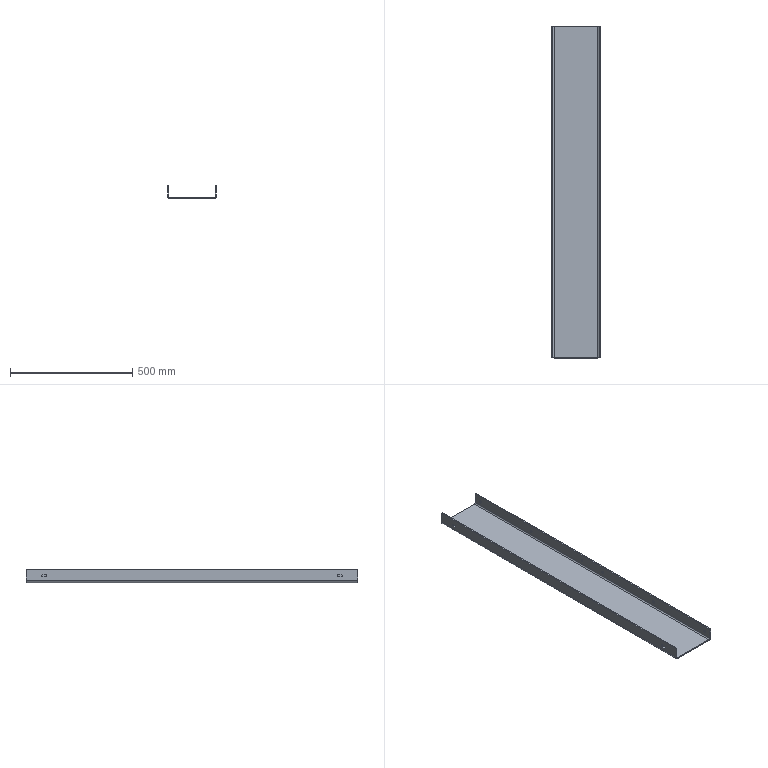Part | STEP file | VD-SYL0380DJ1006_1_1-4_VD-SYL03 | 1 solid | 34 faces | box 200 x 1360 x 55 mm | volume 1991838 mm3 | cylinder 20 | plane 14 | commonest cylinder face diameters 10.5 x12 10 x6 20 x2
STEP:
#1=CARTESIAN_POINT('',(95.,-60.,23.75));
#2=VERTEX_POINT('',#1);
#3=CARTESIAN_POINT('',(100.,-60.,23.75));
#4=VERTEX_POINT('',#3);
#5=CARTESIAN_POINT('',(95.,-60.,23.75));
#6=DIRECTION('',(1.,0.,0.));
#7=VECTOR('',#6,1000.);
#8=LINE('',#5,#7);
#9=EDGE_CURVE('',#2,#4,#8,.T.);
#10=ORIENTED_EDGE('',*,*,#9,.F.);
#11=CARTESIAN_POINT('',(95.,-60.,34.25));
#12=VERTEX_POINT('',#11);
#13=CARTESIAN_POINT('',(95.,-60.,29.));
#14=DIRECTION('',(1.,0.,0.));
#15=DIRECTION('',(0.,0.,1.));
#16=AXIS2_PLACEMENT_3D('',#13,#14,#15);
#17=CIRCLE('',#16,5.25);
#18=EDGE_CURVE('',#12,#2,#17,.T.);
#19=ORIENTED_EDGE('',*,*,#18,.F.);
#20=CARTESIAN_POINT('',(100.,-60.,34.25));
#21=VERTEX_POINT('',#20);
#22=CARTESIAN_POINT('',(95.,-60.,34.25));
#23=DIRECTION('',(1.,0.,0.));
#24=VECTOR('',#23,1000.);
#25=LINE('',#22,#24);
#26=EDGE_CURVE('',#12,#21,#25,.T.);
#27=ORIENTED_EDGE('',*,*,#26,.T.);
#28=CARTESIAN_POINT('',(100.,-60.,29.));
#29=DIRECTION('',(-1.,0.,0.));
#30=DIRECTION('',(0.,0.,-1.));
#31=AXIS2_PLACEMENT_3D('',#28,#29,#30);
#32=CIRCLE('',#31,5.25);
#33=EDGE_CURVE('',#4,#21,#32,.T.);
#34=ORIENTED_EDGE('',*,*,#33,.F.);
#35=EDGE_LOOP('',(#10,#19,#27,#34));
#36=FACE_OUTER_BOUND('',#35,.T.);
#37=CARTESIAN_POINT('',(97.5,-60.,29.));
#38=DIRECTION('',(-1.,0.,0.));
#39=DIRECTION('',(0.,0.,1.));
#40=AXIS2_PLACEMENT_3D('',#37,#38,#39);
#41=CYLINDRICAL_SURFACE('',#40,5.25);
#42=ADVANCED_FACE('',(#36),#41,.F.);
#43=CARTESIAN_POINT('',(100.,-60.,29.));
#44=DIRECTION('',(-1.,0.,0.));
#45=DIRECTION('',(0.,0.,1.));
#46=AXIS2_PLACEMENT_3D('',#43,#44,#45);
#47=CIRCLE('',#46,5.25);
#48=EDGE_CURVE('',#21,#4,#47,.T.);
#49=ORIENTED_EDGE('',*,*,#48,.F.);
#50=ORIENTED_EDGE('',*,*,#26,.F.);
#51=CARTESIAN_POINT('',(95.,-60.,29.));
#52=DIRECTION('',(1.,0.,0.));
#53=DIRECTION('',(0.,0.,-1.));
#54=AXIS2_PLACEMENT_3D('',#51,#52,#53);
#55=CIRCLE('',#54,5.25);
#56=EDGE_CURVE('',#2,#12,#55,.T.);
#57=ORIENTED_EDGE('',*,*,#56,.F.);
#58=ORIENTED_EDGE('',*,*,#9,.T.);
#59=EDGE_LOOP('',(#49,#50,#57,#58));
#60=FACE_OUTER_BOUND('',#59,.T.);
#61=CARTESIAN_POINT('',(97.5,-60.,29.));
#62=DIRECTION('',(-1.,0.,0.));
#63=DIRECTION('',(0.,0.,1.));
#64=AXIS2_PLACEMENT_3D('',#61,#62,#63);
#65=CYLINDRICAL_SURFACE('',#64,5.25);
#66=ADVANCED_FACE('',(#60),#65,.F.);
#67=CARTESIAN_POINT('',(95.,-355.,23.75));
#68=VERTEX_POINT('',#67);
#69=CARTESIAN_POINT('',(100.,-355.,23.75));
#70=VERTEX_POINT('',#69);
#71=CARTESIAN_POINT('',(95.,-355.,23.75));
#72=DIRECTION('',(1.,0.,0.));
#73=VECTOR('',#72,1000.);
#74=LINE('',#71,#73);
#75=EDGE_CURVE('',#68,#70,#74,.T.);
#76=ORIENTED_EDGE('',*,*,#75,.F.);
#77=CARTESIAN_POINT('',(95.,-355.,34.25));
#78=VERTEX_POINT('',#77);
#79=CARTESIAN_POINT('',(95.,-355.,29.));
#80=DIRECTION('',(1.,0.,0.));
#81=DIRECTION('',(0.,0.,1.));
#82=AXIS2_PLACEMENT_3D('',#79,#80,#81);
#83=CIRCLE('',#82,5.25);
#84=EDGE_CURVE('',#78,#68,#83,.T.);
#85=ORIENTED_EDGE('',*,*,#84,.F.);
#86=CARTESIAN_POINT('',(100.,-355.,34.25));
#87=VERTEX_POINT('',#86);
#88=CARTESIAN_POINT('',(95.,-355.,34.25));
#89=DIRECTION('',(1.,0.,0.));
#90=VECTOR('',#89,1000.);
#91=LINE('',#88,#90);
#92=EDGE_CURVE('',#78,#87,#91,.T.);
#93=ORIENTED_EDGE('',*,*,#92,.T.);
#94=CARTESIAN_POINT('',(100.,-355.,29.));
#95=DIRECTION('',(-1.,0.,0.));
#96=DIRECTION('',(0.,0.,-1.));
#97=AXIS2_PLACEMENT_3D('',#94,#95,#96);
#98=CIRCLE('',#97,5.25);
#99=EDGE_CURVE('',#70,#87,#98,.T.);
#100=ORIENTED_EDGE('',*,*,#99,.F.);
#101=EDGE_LOOP('',(#76,#85,#93,#100));
#102=FACE_OUTER_BOUND('',#101,.T.);
#103=CARTESIAN_POINT('',(97.5,-355.,29.));
#104=DIRECTION('',(-1.,0.,0.));
#105=DIRECTION('',(0.,0.,1.));
#106=AXIS2_PLACEMENT_3D('',#103,#104,#105);
#107=CYLINDRICAL_SURFACE('',#106,5.25);
#108=ADVANCED_FACE('',(#102),#107,.F.);
#109=CARTESIAN_POINT('',(100.,-355.,29.));
#110=DIRECTION('',(-1.,0.,0.));
#111=DIRECTION('',(0.,0.,1.));
#112=AXIS2_PLACEMENT_3D('',#109,#110,#111);
#113=CIRCLE('',#112,5.25);
#114=EDGE_CURVE('',#87,#70,#113,.T.);
#115=ORIENTED_EDGE('',*,*,#114,.F.);
#116=ORIENTED_EDGE('',*,*,#92,.F.);
#117=CARTESIAN_POINT('',(95.,-355.,29.));
#118=DIRECTION('',(1.,0.,0.));
#119=DIRECTION('',(0.,0.,-1.));
#120=AXIS2_PLACEMENT_3D('',#117,#118,#119);
#121=CIRCLE('',#120,5.25);
#122=EDGE_CURVE('',#68,#78,#121,.T.);
#123=ORIENTED_EDGE('',*,*,#122,.F.);
#124=ORIENTED_EDGE('',*,*,#75,.T.);
#125=EDGE_LOOP('',(#115,#116,#123,#124));
#126=FACE_OUTER_BOUND('',#125,.T.);
#127=CARTESIAN_POINT('',(97.5,-355.,29.));
#128=DIRECTION('',(-1.,0.,0.));
#129=DIRECTION('',(0.,0.,1.));
#130=AXIS2_PLACEMENT_3D('',#127,#128,#129);
#131=CYLINDRICAL_SURFACE('',#130,5.25);
#132=ADVANCED_FACE('',(#126),#131,.F.);
#133=CARTESIAN_POINT('',(95.,-650.,23.75));
#134=VERTEX_POINT('',#133);
#135=CARTESIAN_POINT('',(100.,-650.,23.75));
#136=VERTEX_POINT('',#135);
#137=CARTESIAN_POINT('',(95.,-650.,23.75));
#138=DIRECTION('',(1.,0.,0.));
#139=VECTOR('',#138,1000.);
#140=LINE('',#137,#139);
#141=EDGE_CURVE('',#134,#136,#140,.T.);
#142=ORIENTED_EDGE('',*,*,#141,.F.);
#143=CARTESIAN_POINT('',(95.,-650.,34.25));
#144=VERTEX_POINT('',#143);
#145=CARTESIAN_POINT('',(95.,-650.,29.));
#146=DIRECTION('',(1.,0.,0.));
#147=DIRECTION('',(0.,0.,1.));
#148=AXIS2_PLACEMENT_3D('',#145,#146,#147);
#149=CIRCLE('',#148,5.25);
#150=EDGE_CURVE('',#144,#134,#149,.T.);
#151=ORIENTED_EDGE('',*,*,#150,.F.);
#152=CARTESIAN_POINT('',(100.,-650.,34.25));
#153=VERTEX_POINT('',#152);
#154=CARTESIAN_POINT('',(95.,-650.,34.25));
#155=DIRECTION('',(1.,0.,0.));
#156=VECTOR('',#155,1000.);
#157=LINE('',#154,#156);
#158=EDGE_CURVE('',#144,#153,#157,.T.);
#159=ORIENTED_EDGE('',*,*,#158,.T.);
#160=CARTESIAN_POINT('',(100.,-650.,29.));
#161=DIRECTION('',(-1.,0.,0.));
#162=DIRECTION('',(0.,0.,-1.));
#163=AXIS2_PLACEMENT_3D('',#160,#161,#162);
#164=CIRCLE('',#163,5.25);
#165=EDGE_CURVE('',#136,#153,#164,.T.);
#166=ORIENTED_EDGE('',*,*,#165,.F.);
#167=EDGE_LOOP('',(#142,#151,#159,#166));
#168=FACE_OUTER_BOUND('',#167,.T.);
#169=CARTESIAN_POINT('',(97.5,-650.,29.));
#170=DIRECTION('',(-1.,0.,0.));
#171=DIRECTION('',(0.,0.,1.));
#172=AXIS2_PLACEMENT_3D('',#169,#170,#171);
#173=CYLINDRICAL_SURFACE('',#172,5.25);
#174=ADVANCED_FACE('',(#168),#173,.F.);
#175=CARTESIAN_POINT('',(100.,-650.,29.));
#176=DIRECTION('',(-1.,0.,0.));
#177=DIRECTION('',(0.,0.,1.));
#178=AXIS2_PLACEMENT_3D('',#175,#176,#177);
#179=CIRCLE('',#178,5.25);
#180=EDGE_CURVE('',#153,#136,#179,.T.);
#181=ORIENTED_EDGE('',*,*,#180,.F.);
#182=ORIENTED_EDGE('',*,*,#158,.F.);
#183=CARTESIAN_POINT('',(95.,-650.,29.));
#184=DIRECTION('',(1.,0.,0.));
#185=DIRECTION('',(0.,0.,-1.));
#186=AXIS2_PLACEMENT_3D('',#183,#184,#185);
#187=CIRCLE('',#186,5.25);
#188=EDGE_CURVE('',#134,#144,#187,.T.);
#189=ORIENTED_EDGE('',*,*,#188,.F.);
#190=ORIENTED_EDGE('',*,*,#141,.T.);
#191=EDGE_LOOP('',(#181,#182,#189,#190));
#192=FACE_OUTER_BOUND('',#191,.T.);
#193=CARTESIAN_POINT('',(97.5,-650.,29.));
#194=DIRECTION('',(-1.,0.,0.));
#195=DIRECTION('',(0.,0.,1.));
#196=AXIS2_PLACEMENT_3D('',#193,#194,#195);
#197=CYLINDRICAL_SURFACE('',#196,5.25);
#198=ADVANCED_FACE('',(#192),#197,.F.);
#199=CARTESIAN_POINT('',(95.,60.,23.75));
#200=VERTEX_POINT('',#199);
#201=CARTESIAN_POINT('',(95.,60.,34.25));
#202=VERTEX_POINT('',#201);
#203=CARTESIAN_POINT('',(95.,60.,29.));
#204=DIRECTION('',(1.,0.,0.));
#205=DIRECTION('',(0.,0.,-1.));
#206=AXIS2_PLACEMENT_3D('',#203,#204,#205);
#207=CIRCLE('',#206,5.25);
#208=EDGE_CURVE('',#200,#202,#207,.T.);
#209=ORIENTED_EDGE('',*,*,#208,.F.);
#210=CARTESIAN_POINT('',(100.,60.,23.75));
#211=VERTEX_POINT('',#210);
#212=CARTESIAN_POINT('',(100.,60.,23.75));
#213=DIRECTION('',(-1.,0.,0.));
#214=VECTOR('',#213,1000.);
#215=LINE('',#212,#214);
#216=EDGE_CURVE('',#211,#200,#215,.T.);
#217=ORIENTED_EDGE('',*,*,#216,.F.);
#218=CARTESIAN_POINT('',(100.,60.,34.25));
#219=VERTEX_POINT('',#218);
#220=CARTESIAN_POINT('',(100.,60.,29.));
#221=DIRECTION('',(-1.,0.,0.));
#222=DIRECTION('',(0.,0.,1.));
#223=AXIS2_PLACEMENT_3D('',#220,#221,#222);
#224=CIRCLE('',#223,5.25);
#225=EDGE_CURVE('',#219,#211,#224,.T.);
#226=ORIENTED_EDGE('',*,*,#225,.F.);
#227=CARTESIAN_POINT('',(100.,60.,34.25));
#228=DIRECTION('',(-1.,0.,0.));
#229=VECTOR('',#228,1000.);
#230=LINE('',#227,#229);
#231=EDGE_CURVE('',#219,#202,#230,.T.);
#232=ORIENTED_EDGE('',*,*,#231,.T.);
#233=EDGE_LOOP('',(#209,#217,#226,#232));
#234=FACE_OUTER_BOUND('',#233,.T.);
#235=CARTESIAN_POINT('',(97.5,60.,29.));
#236=DIRECTION('',(1.,0.,0.));
#237=DIRECTION('',(0.,0.,-1.));
#238=AXIS2_PLACEMENT_3D('',#235,#236,#237);
#239=CYLINDRICAL_SURFACE('',#238,5.25);
#240=ADVANCED_FACE('',(#234),#239,.F.);
#241=ORIENTED_EDGE('',*,*,#231,.F.);
#242=CARTESIAN_POINT('',(100.,60.,29.));
#243=DIRECTION('',(-1.,0.,0.));
#244=DIRECTION('',(0.,0.,-1.));
#245=AXIS2_PLACEMENT_3D('',#242,#243,#244);
#246=CIRCLE('',#245,5.25);
#247=EDGE_CURVE('',#211,#219,#246,.T.);
#248=ORIENTED_EDGE('',*,*,#247,.F.);
#249=ORIENTED_EDGE('',*,*,#216,.T.);
#250=CARTESIAN_POINT('',(95.,60.,29.));
#251=DIRECTION('',(1.,0.,0.));
#252=DIRECTION('',(0.,0.,1.));
#253=AXIS2_PLACEMENT_3D('',#250,#251,#252);
#254=CIRCLE('',#253,5.25);
#255=EDGE_CURVE('',#202,#200,#254,.T.);
#256=ORIENTED_EDGE('',*,*,#255,.F.);
#257=EDGE_LOOP('',(#241,#248,#249,#256));
#258=FACE_OUTER_BOUND('',#257,.T.);
#259=CARTESIAN_POINT('',(97.5,60.,29.));
#260=DIRECTION('',(1.,0.,0.));
#261=DIRECTION('',(0.,0.,-1.));
#262=AXIS2_PLACEMENT_3D('',#259,#260,#261);
#263=CYLINDRICAL_SURFACE('',#262,5.25);
#264=ADVANCED_FACE('',(#258),#263,.F.);
#265=CARTESIAN_POINT('',(95.,355.,23.75));
#266=VERTEX_POINT('',#265);
#267=CARTESIAN_POINT('',(95.,355.,34.25));
#268=VERTEX_POINT('',#267);
#269=CARTESIAN_POINT('',(95.,355.,29.));
#270=DIRECTION('',(1.,0.,0.));
#271=DIRECTION('',(0.,0.,-1.));
#272=AXIS2_PLACEMENT_3D('',#269,#270,#271);
#273=CIRCLE('',#272,5.25);
#274=EDGE_CURVE('',#266,#268,#273,.T.);
#275=ORIENTED_EDGE('',*,*,#274,.F.);
#276=CARTESIAN_POINT('',(100.,355.,23.75));
#277=VERTEX_POINT('',#276);
#278=CARTESIAN_POINT('',(100.,355.,23.75));
#279=DIRECTION('',(-1.,0.,0.));
#280=VECTOR('',#279,1000.);
#281=LINE('',#278,#280);
#282=EDGE_CURVE('',#277,#266,#281,.T.);
#283=ORIENTED_EDGE('',*,*,#282,.F.);
#284=CARTESIAN_POINT('',(100.,355.,34.25));
#285=VERTEX_POINT('',#284);
#286=CARTESIAN_POINT('',(100.,355.,29.));
#287=DIRECTION('',(-1.,0.,0.));
#288=DIRECTION('',(0.,0.,1.));
#289=AXIS2_PLACEMENT_3D('',#286,#287,#288);
#290=CIRCLE('',#289,5.25);
#291=EDGE_CURVE('',#285,#277,#290,.T.);
#292=ORIENTED_EDGE('',*,*,#291,.F.);
#293=CARTESIAN_POINT('',(100.,355.,34.25));
#294=DIRECTION('',(-1.,0.,0.));
#295=VECTOR('',#294,1000.);
#296=LINE('',#293,#295);
#297=EDGE_CURVE('',#285,#268,#296,.T.);
#298=ORIENTED_EDGE('',*,*,#297,.T.);
#299=EDGE_LOOP('',(#275,#283,#292,#298));
#300=FACE_OUTER_BOUND('',#299,.T.);
#301=CARTESIAN_POINT('',(97.5,355.,29.));
#302=DIRECTION('',(1.,0.,0.));
#303=DIRECTION('',(0.,0.,-1.));
#304=AXIS2_PLACEMENT_3D('',#301,#302,#303);
#305=CYLINDRICAL_SURFACE('',#304,5.25);
#306=ADVANCED_FACE('',(#300),#305,.F.);
#307=ORIENTED_EDGE('',*,*,#297,.F.);
#308=CARTESIAN_POINT('',(100.,355.,29.));
#309=DIRECTION('',(-1.,0.,0.));
#310=DIRECTION('',(0.,0.,-1.));
#311=AXIS2_PLACEMENT_3D('',#308,#309,#310);
#312=CIRCLE('',#311,5.25);
#313=EDGE_CURVE('',#277,#285,#312,.T.);
#314=ORIENTED_EDGE('',*,*,#313,.F.);
#315=ORIENTED_EDGE('',*,*,#282,.T.);
#316=CARTESIAN_POINT('',(95.,355.,29.));
#317=DIRECTION('',(1.,0.,0.));
#318=DIRECTION('',(0.,0.,1.));
#319=AXIS2_PLACEMENT_3D('',#316,#317,#318);
#320=CIRCLE('',#319,5.25);
#321=EDGE_CURVE('',#268,#266,#320,.T.);
#322=ORIENTED_EDGE('',*,*,#321,.F.);
#323=EDGE_LOOP('',(#307,#314,#315,#322));
#324=FACE_OUTER_BOUND('',#323,.T.);
#325=CARTESIAN_POINT('',(97.5,355.,29.));
#326=DIRECTION('',(1.,0.,0.));
#327=DIRECTION('',(0.,0.,-1.));
#328=AXIS2_PLACEMENT_3D('',#325,#326,#327);
#329=CYLINDRICAL_SURFACE('',#328,5.25);
#330=ADVANCED_FACE('',(#324),#329,.F.);
#331=CARTESIAN_POINT('',(95.,650.,23.75));
#332=VERTEX_POINT('',#331);
#333=CARTESIAN_POINT('',(95.,650.,34.25));
#334=VERTEX_POINT('',#333);
#335=CARTESIAN_POINT('',(95.,650.,29.));
#336=DIRECTION('',(1.,0.,0.));
#337=DIRECTION('',(0.,0.,-1.));
#338=AXIS2_PLACEMENT_3D('',#335,#336,#337);
#339=CIRCLE('',#338,5.25);
#340=EDGE_CURVE('',#332,#334,#339,.T.);
#341=ORIENTED_EDGE('',*,*,#340,.F.);
#342=CARTESIAN_POINT('',(100.,650.,23.75));
#343=VERTEX_POINT('',#342);
#344=CARTESIAN_POINT('',(100.,650.,23.75));
#345=DIRECTION('',(-1.,0.,0.));
#346=VECTOR('',#345,1000.);
#347=LINE('',#344,#346);
#348=EDGE_CURVE('',#343,#332,#347,.T.);
#349=ORIENTED_EDGE('',*,*,#348,.F.);
#350=CARTESIAN_POINT('',(100.,650.,34.25));
#351=VERTEX_POINT('',#350);
#352=CARTESIAN_POINT('',(100.,650.,29.));
#353=DIRECTION('',(-1.,0.,0.));
#354=DIRECTION('',(0.,0.,1.));
#355=AXIS2_PLACEMENT_3D('',#352,#353,#354);
#356=CIRCLE('',#355,5.25);
#357=EDGE_CURVE('',#351,#343,#356,.T.);
#358=ORIENTED_EDGE('',*,*,#357,.F.);
#359=CARTESIAN_POINT('',(100.,650.,34.25));
#360=DIRECTION('',(-1.,0.,0.));
#361=VECTOR('',#360,1000.);
#362=LINE('',#359,#361);
#363=EDGE_CURVE('',#351,#334,#362,.T.);
#364=ORIENTED_EDGE('',*,*,#363,.T.);
#365=EDGE_LOOP('',(#341,#349,#358,#364));
#366=FACE_OUTER_BOUND('',#365,.T.);
#367=CARTESIAN_POINT('',(97.5,650.,29.));
#368=DIRECTION('',(1.,0.,0.));
#369=DIRECTION('',(0.,0.,-1.));
#370=AXIS2_PLACEMENT_3D('',#367,#368,#369);
#371=CYLINDRICAL_SURFACE('',#370,5.25);
#372=ADVANCED_FACE('',(#366),#371,.F.);
#373=ORIENTED_EDGE('',*,*,#363,.F.);
#374=CARTESIAN_POINT('',(100.,650.,29.));
#375=DIRECTION('',(-1.,0.,0.));
#376=DIRECTION('',(0.,0.,-1.));
#377=AXIS2_PLACEMENT_3D('',#374,#375,#376);
#378=CIRCLE('',#377,5.25);
#379=EDGE_CURVE('',#343,#351,#378,.T.);
#380=ORIENTED_EDGE('',*,*,#379,.F.);
#381=ORIENTED_EDGE('',*,*,#348,.T.);
#382=CARTESIAN_POINT('',(95.,650.,29.));
#383=DIRECTION('',(1.,0.,0.));
#384=DIRECTION('',(0.,0.,1.));
#385=AXIS2_PLACEMENT_3D('',#382,#383,#384);
#386=CIRCLE('',#385,5.25);
#387=EDGE_CURVE('',#334,#332,#386,.T.);
#388=ORIENTED_EDGE('',*,*,#387,.F.);
#389=EDGE_LOOP('',(#373,#380,#381,#388));
#390=FACE_OUTER_BOUND('',#389,.T.);
#391=CARTESIAN_POINT('',(97.5,650.,29.));
#392=DIRECTION('',(1.,0.,0.));
#393=DIRECTION('',(0.,0.,-1.));
#394=AXIS2_PLACEMENT_3D('',#391,#392,#393);
#395=CYLINDRICAL_SURFACE('',#394,5.25);
#396=ADVANCED_FACE('',(#390),#395,.F.);
#397=CARTESIAN_POINT('',(-95.,-601.,33.5));
#398=VERTEX_POINT('',#397);
#399=CARTESIAN_POINT('',(-100.,-601.,33.5));
#400=VERTEX_POINT('',#399);
#401=CARTESIAN_POINT('',(-95.,-601.,33.5));
#402=DIRECTION('',(-1.,0.,0.));
#403=VECTOR('',#402,1000.);
#404=LINE('',#401,#403);
#405=EDGE_CURVE('',#398,#400,#404,.T.);
#406=ORIENTED_EDGE('',*,*,#405,.T.);
#407=CARTESIAN_POINT('',(-100.,-601.,23.5));
#408=VERTEX_POINT('',#407);
#409=CARTESIAN_POINT('',(-100.,-601.,28.5));
#410=DIRECTION('',(1.,0.,0.));
#411=DIRECTION('',(0.,0.,-1.));
#412=AXIS2_PLACEMENT_3D('',#409,#410,#411);
#413=CIRCLE('',#412,5.);
#414=EDGE_CURVE('',#408,#400,#413,.T.);
#415=ORIENTED_EDGE('',*,*,#414,.F.);
#416=CARTESIAN_POINT('',(-95.,-601.,23.5));
#417=VERTEX_POINT('',#416);
#418=CARTESIAN_POINT('',(-100.,-601.,23.5));
#419=DIRECTION('',(1.,0.,0.));
#420=VECTOR('',#419,1000.);
#421=LINE('',#418,#420);
#422=EDGE_CURVE('',#408,#417,#421,.T.);
#423=ORIENTED_EDGE('',*,*,#422,.T.);
#424=CARTESIAN_POINT('',(-95.,-601.,28.5));
#425=DIRECTION('',(-1.,0.,0.));
#426=DIRECTION('',(0.,0.,1.));
#427=AXIS2_PLACEMENT_3D('',#424,#425,#426);
#428=CIRCLE('',#427,5.);
#429=EDGE_CURVE('',#398,#417,#428,.T.);
#430=ORIENTED_EDGE('',*,*,#429,.F.);
#431=EDGE_LOOP('',(#406,#415,#423,#430));
#432=FACE_OUTER_BOUND('',#431,.T.);
#433=CARTESIAN_POINT('',(-97.5,-601.,28.5));
#434=DIRECTION('',(-1.,0.,0.));
#435=DIRECTION('',(0.,0.,1.));
#436=AXIS2_PLACEMENT_3D('',#433,#434,#435);
#437=CYLINDRICAL_SURFACE('',#436,5.);
#438=ADVANCED_FACE('',(#432),#437,.F.);
#439=CARTESIAN_POINT('',(-100.,-611.,23.5));
#440=VERTEX_POINT('',#439);
#441=CARTESIAN_POINT('',(-100.,-601.,23.5));
#442=DIRECTION('',(0.,-1.,0.));
#443=VECTOR('',#442,1000.);
#444=LINE('',#441,#443);
#445=EDGE_CURVE('',#408,#440,#444,.T.);
#446=ORIENTED_EDGE('',*,*,#445,.T.);
#447=CARTESIAN_POINT('',(-95.,-611.,23.5));
#448=VERTEX_POINT('',#447);
#449=CARTESIAN_POINT('',(-95.,-611.,23.5));
#450=DIRECTION('',(-1.,0.,0.));
#451=VECTOR('',#450,1000.);
#452=LINE('',#449,#451);
#453=EDGE_CURVE('',#448,#440,#452,.T.);
#454=ORIENTED_EDGE('',*,*,#453,.F.);
#455=CARTESIAN_POINT('',(-95.,-601.,23.5));
#456=DIRECTION('',(0.,-1.,0.));
#457=VECTOR('',#456,1000.);
#458=LINE('',#455,#457);
#459=EDGE_CURVE('',#417,#448,#458,.T.);
#460=ORIENTED_EDGE('',*,*,#459,.F.);
#461=ORIENTED_EDGE('',*,*,#422,.F.);
#462=EDGE_LOOP('',(#446,#454,#460,#461));
#463=FACE_OUTER_BOUND('',#462,.T.);
#464=CARTESIAN_POINT('',(-97.5,-606.,23.5));
#465=DIRECTION('',(0.,0.,1.));
#466=DIRECTION('',(1.,0.,0.));
#467=AXIS2_PLACEMENT_3D('',#464,#465,#466);
#468=PLANE('',#467);
#469=ADVANCED_FACE('',(#463),#468,.T.);
#470=ORIENTED_EDGE('',*,*,#453,.T.);
#471=CARTESIAN_POINT('',(-100.,-611.,33.5));
#472=VERTEX_POINT('',#471);
#473=CARTESIAN_POINT('',(-100.,-611.,28.5));
#474=DIRECTION('',(1.,0.,0.));
#475=DIRECTION('',(0.,0.,1.));
#476=AXIS2_PLACEMENT_3D('',#473,#474,#475);
#477=CIRCLE('',#476,5.);
#478=EDGE_CURVE('',#472,#440,#477,.T.);
#479=ORIENTED_EDGE('',*,*,#478,.F.);
#480=CARTESIAN_POINT('',(-95.,-611.,33.5));
#481=VERTEX_POINT('',#480);
#482=CARTESIAN_POINT('',(-100.,-611.,33.5));
#483=DIRECTION('',(1.,0.,0.));
#484=VECTOR('',#483,1000.);
#485=LINE('',#482,#484);
#486=EDGE_CURVE('',#472,#481,#485,.T.);
#487=ORIENTED_EDGE('',*,*,#486,.T.);
#488=CARTESIAN_POINT('',(-95.,-611.,28.5));
#489=DIRECTION('',(-1.,0.,0.));
#490=DIRECTION('',(0.,0.,-1.));
#491=AXIS2_PLACEMENT_3D('',#488,#489,#490);
#492=CIRCLE('',#491,5.);
#493=EDGE_CURVE('',#448,#481,#492,.T.);
#494=ORIENTED_EDGE('',*,*,#493,.F.);
#495=EDGE_LOOP('',(#470,#479,#487,#494));
#496=FACE_OUTER_BOUND('',#495,.T.);
#497=CARTESIAN_POINT('',(-97.5,-611.,28.5));
#498=DIRECTION('',(-1.,0.,0.));
#499=DIRECTION('',(0.,0.,1.));
#500=AXIS2_PLACEMENT_3D('',#497,#498,#499);
#501=CYLINDRICAL_SURFACE('',#500,5.);
#502=ADVANCED_FACE('',(#496),#501,.F.);
#503=CARTESIAN_POINT('',(-100.,-611.,33.5));
#504=DIRECTION('',(0.,1.,0.));
#505=VECTOR('',#504,1000.);
#506=LINE('',#503,#505);
#507=EDGE_CURVE('',#472,#400,#506,.T.);
#508=ORIENTED_EDGE('',*,*,#507,.T.);
#509=ORIENTED_EDGE('',*,*,#405,.F.);
#510=CARTESIAN_POINT('',(-95.,-611.,33.5));
#511=DIRECTION('',(0.,1.,0.));
#512=VECTOR('',#511,1000.);
#513=LINE('',#510,#512);
#514=EDGE_CURVE('',#481,#398,#513,.T.);
#515=ORIENTED_EDGE('',*,*,#514,.F.);
#516=ORIENTED_EDGE('',*,*,#486,.F.);
#517=EDGE_LOOP('',(#508,#509,#515,#516));
#518=FACE_OUTER_BOUND('',#517,.T.);
#519=CARTESIAN_POINT('',(-97.5,-606.,33.5));
#520=DIRECTION('',(0.,0.,-1.));
#521=DIRECTION('',(0.,-1.,0.));
#522=AXIS2_PLACEMENT_3D('',#519,#520,#521);
#523=PLANE('',#522);
#524=ADVANCED_FACE('',(#518),#523,.T.);
#525=CARTESIAN_POINT('',(-100.,611.,23.5));
#526=VERTEX_POINT('',#525);
#527=CARTESIAN_POINT('',(-100.,601.,23.5));
#528=VERTEX_POINT('',#527);
#529=CARTESIAN_POINT('',(-100.,611.,23.5));
#530=DIRECTION('',(0.,-1.,0.));
#531=VECTOR('',#530,1000.);
#532=LINE('',#529,#531);
#533=EDGE_CURVE('',#526,#528,#532,.T.);
#534=ORIENTED_EDGE('',*,*,#533,.T.);
#535=CARTESIAN_POINT('',(-95.,601.,23.5));
#536=VERTEX_POINT('',#535);
#537=CARTESIAN_POINT('',(-95.,601.,23.5));
#538=DIRECTION('',(-1.,0.,0.));
#539=VECTOR('',#538,1000.);
#540=LINE('',#537,#539);
#541=EDGE_CURVE('',#536,#528,#540,.T.);
#542=ORIENTED_EDGE('',*,*,#541,.F.);
#543=CARTESIAN_POINT('',(-95.,611.,23.5));
#544=VERTEX_POINT('',#543);
#545=CARTESIAN_POINT('',(-95.,611.,23.5));
#546=DIRECTION('',(0.,-1.,0.));
#547=VECTOR('',#546,1000.);
#548=LINE('',#545,#547);
#549=EDGE_CURVE('',#544,#536,#548,.T.);
#550=ORIENTED_EDGE('',*,*,#549,.F.);
#551=CARTESIAN_POINT('',(-100.,611.,23.5));
#552=DIRECTION('',(1.,0.,0.));
#553=VECTOR('',#552,1000.);
#554=LINE('',#551,#553);
#555=EDGE_CURVE('',#526,#544,#554,.T.);
#556=ORIENTED_EDGE('',*,*,#555,.F.);
#557=EDGE_LOOP('',(#534,#542,#550,#556));
#558=FACE_OUTER_BOUND('',#557,.T.);
#559=CARTESIAN_POINT('',(-97.5,606.,23.5));
#560=DIRECTION('',(0.,0.,1.));
#561=DIRECTION('',(1.,0.,0.));
#562=AXIS2_PLACEMENT_3D('',#559,#560,#561);
#563=PLANE('',#562);
#564=ADVANCED_FACE('',(#558),#563,.T.);
#565=CARTESIAN_POINT('',(-95.,611.,33.5));
#566=VERTEX_POINT('',#565);
#567=CARTESIAN_POINT('',(-100.,611.,33.5));
#568=VERTEX_POINT('',#567);
#569=CARTESIAN_POINT('',(-95.,611.,33.5));
#570=DIRECTION('',(-1.,0.,0.));
#571=VECTOR('',#570,1000.);
#572=LINE('',#569,#571);
#573=EDGE_CURVE('',#566,#568,#572,.T.);
#574=ORIENTED_EDGE('',*,*,#573,.T.);
#575=CARTESIAN_POINT('',(-100.,611.,28.5));
#576=DIRECTION('',(1.,0.,0.));
#577=DIRECTION('',(0.,0.,-1.));
#578=AXIS2_PLACEMENT_3D('',#575,#576,#577);
#579=CIRCLE('',#578,5.);
#580=EDGE_CURVE('',#526,#568,#579,.T.);
#581=ORIENTED_EDGE('',*,*,#580,.F.);
#582=ORIENTED_EDGE('',*,*,#555,.T.);
#583=CARTESIAN_POINT('',(-95.,611.,28.5));
#584=DIRECTION('',(-1.,0.,0.));
#585=DIRECTION('',(0.,0.,1.));
#586=AXIS2_PLACEMENT_3D('',#583,#584,#585);
#587=CIRCLE('',#586,5.);
#588=EDGE_CURVE('',#566,#544,#587,.T.);
#589=ORIENTED_EDGE('',*,*,#588,.F.);
#590=EDGE_LOOP('',(#574,#581,#582,#589));
#591=FACE_OUTER_BOUND('',#590,.T.);
#592=CARTESIAN_POINT('',(-97.5,611.,28.5));
#593=DIRECTION('',(-1.,0.,0.));
#594=DIRECTION('',(0.,0.,1.));
#595=AXIS2_PLACEMENT_3D('',#592,#593,#594);
#596=CYLINDRICAL_SURFACE('',#595,5.);
#597=ADVANCED_FACE('',(#591),#596,.F.);
#598=CARTESIAN_POINT('',(-100.,601.,33.5));
#599=VERTEX_POINT('',#598);
#600=CARTESIAN_POINT('',(-100.,601.,33.5));
#601=DIRECTION('',(0.,1.,0.));
#602=VECTOR('',#601,1000.);
#603=LINE('',#600,#602);
#604=EDGE_CURVE('',#599,#568,#603,.T.);
#605=ORIENTED_EDGE('',*,*,#604,.T.);
#606=ORIENTED_EDGE('',*,*,#573,.F.);
#607=CARTESIAN_POINT('',(-95.,601.,33.5));
#608=VERTEX_POINT('',#607);
#609=CARTESIAN_POINT('',(-95.,601.,33.5));
#610=DIRECTION('',(0.,1.,0.));
#611=VECTOR('',#610,1000.);
#612=LINE('',#609,#611);
#613=EDGE_CURVE('',#608,#566,#612,.T.);
#614=ORIENTED_EDGE('',*,*,#613,.F.);
#615=CARTESIAN_POINT('',(-100.,601.,33.5));
#616=DIRECTION('',(1.,0.,0.));
#617=VECTOR('',#616,1000.);
#618=LINE('',#615,#617);
#619=EDGE_CURVE('',#599,#608,#618,.T.);
#620=ORIENTED_EDGE('',*,*,#619,.F.);
#621=EDGE_LOOP('',(#605,#606,#614,#620));
#622=FACE_OUTER_BOUND('',#621,.T.);
#623=CARTESIAN_POINT('',(-97.5,606.,33.5));
#624=DIRECTION('',(0.,0.,-1.));
#625=DIRECTION('',(0.,-1.,0.));
#626=AXIS2_PLACEMENT_3D('',#623,#624,#625);
#627=PLANE('',#626);
#628=ADVANCED_FACE('',(#622),#627,.T.);
#629=CARTESIAN_POINT('',(-95.,680.,10.));
#630=VERTEX_POINT('',#629);
#631=CARTESIAN_POINT('',(-90.,680.,5.));
#632=VERTEX_POINT('',#631);
#633=CARTESIAN_POINT('',(-90.,680.,10.));
#634=DIRECTION('',(0.,-1.,0.));
#635=DIRECTION('',(-1.,0.,0.));
#636=AXIS2_PLACEMENT_3D('',#633,#634,#635);
#637=CIRCLE('',#636,5.);
#638=EDGE_CURVE('',#630,#632,#637,.T.);
#639=ORIENTED_EDGE('',*,*,#638,.F.);
#640=CARTESIAN_POINT('',(-95.,-680.,10.));
#641=VERTEX_POINT('',#640);
#642=CARTESIAN_POINT('',(-95.,680.,10.));
#643=DIRECTION('',(0.,-1.,0.));
#644=VECTOR('',#643,1000.);
#645=LINE('',#642,#644);
#646=EDGE_CURVE('',#630,#641,#645,.T.);
#647=ORIENTED_EDGE('',*,*,#646,.T.);
#648=CARTESIAN_POINT('',(-90.,-680.,5.));
#649=VERTEX_POINT('',#648);
#650=CARTESIAN_POINT('',(-90.,-680.,10.));
#651=DIRECTION('',(0.,1.,0.));
#652=DIRECTION('',(0.,0.,-1.));
#653=AXIS2_PLACEMENT_3D('',#650,#651,#652);
#654=CIRCLE('',#653,5.);
#655=EDGE_CURVE('',#649,#641,#654,.T.);
#656=ORIENTED_EDGE('',*,*,#655,.F.);
#657=CARTESIAN_POINT('',(-90.,-680.,5.));
#658=DIRECTION('',(0.,1.,0.));
#659=VECTOR('',#658,1000.);
#660=LINE('',#657,#659);
#661=EDGE_CURVE('',#649,#632,#660,.T.);
#662=ORIENTED_EDGE('',*,*,#661,.T.);
#663=EDGE_LOOP('',(#639,#647,#656,#662));
#664=FACE_OUTER_BOUND('',#663,.T.);
#665=CARTESIAN_POINT('',(-90.,680.,10.));
#666=DIRECTION('',(0.,-1.,0.));
#667=DIRECTION('',(0.,0.,-1.));
#668=AXIS2_PLACEMENT_3D('',#665,#666,#667);
#669=CYLINDRICAL_SURFACE('',#668,5.);
#670=ADVANCED_FACE('',(#664),#669,.F.);
#671=ORIENTED_EDGE('',*,*,#429,.T.);
#672=ORIENTED_EDGE('',*,*,#459,.T.);
#673=ORIENTED_EDGE('',*,*,#493,.T.);
#674=ORIENTED_EDGE('',*,*,#514,.T.);
#675=EDGE_LOOP('',(#671,#672,#673,#674));
#676=FACE_BOUND('',#675,.T.);
#677=ORIENTED_EDGE('',*,*,#588,.T.);
#678=ORIENTED_EDGE('',*,*,#549,.T.);
#679=CARTESIAN_POINT('',(-95.,601.,28.5));
#680=DIRECTION('',(-1.,0.,0.));
#681=DIRECTION('',(0.,0.,-1.));
#682=AXIS2_PLACEMENT_3D('',#679,#680,#681);
#683=CIRCLE('',#682,5.);
#684=EDGE_CURVE('',#536,#608,#683,.T.);
#685=ORIENTED_EDGE('',*,*,#684,.T.);
#686=ORIENTED_EDGE('',*,*,#613,.T.);
#687=EDGE_LOOP('',(#677,#678,#685,#686));
#688=FACE_BOUND('',#687,.T.);
#689=CARTESIAN_POINT('',(-95.,680.,55.));
#690=VERTEX_POINT('',#689);
#691=CARTESIAN_POINT('',(-95.,-680.,55.));
#692=VERTEX_POINT('',#691);
#693=CARTESIAN_POINT('',(-95.,680.,55.));
#694=DIRECTION('',(0.,-1.,0.));
#695=VECTOR('',#694,1000.);
#696=LINE('',#693,#695);
#697=EDGE_CURVE('',#690,#692,#696,.T.);
#698=ORIENTED_EDGE('',*,*,#697,.T.);
#699=CARTESIAN_POINT('',(-95.,-680.,55.));
#700=DIRECTION('',(0.,0.,-1.));
#701=VECTOR('',#700,1000.);
#702=LINE('',#699,#701);
#703=EDGE_CURVE('',#692,#641,#702,.T.);
#704=ORIENTED_EDGE('',*,*,#703,.T.);
#705=ORIENTED_EDGE('',*,*,#646,.F.);
#706=CARTESIAN_POINT('',(-95.,680.,10.));
#707=DIRECTION('',(0.,0.,1.));
#708=VECTOR('',#707,1000.);
#709=LINE('',#706,#708);
#710=EDGE_CURVE('',#630,#690,#709,.T.);
#711=ORIENTED_EDGE('',*,*,#710,.T.);
#712=EDGE_LOOP('',(#698,#704,#705,#711));
#713=FACE_OUTER_BOUND('',#712,.T.);
#714=CARTESIAN_POINT('',(-95.,-680.,0.));
#715=DIRECTION('',(-1.,0.,0.));
#716=DIRECTION('',(0.,0.,1.));
#717=AXIS2_PLACEMENT_3D('',#714,#715,#716);
#718=PLANE('',#717);
#719=ADVANCED_FACE('',(#676,#688,#713),#718,.F.);
#720=ORIENTED_EDGE('',*,*,#541,.T.);
#721=CARTESIAN_POINT('',(-100.,601.,28.5));
#722=DIRECTION('',(1.,0.,0.));
#723=DIRECTION('',(0.,0.,1.));
#724=AXIS2_PLACEMENT_3D('',#721,#722,#723);
#725=CIRCLE('',#724,5.);
#726=EDGE_CURVE('',#599,#528,#725,.T.);
#727=ORIENTED_EDGE('',*,*,#726,.F.);
#728=ORIENTED_EDGE('',*,*,#619,.T.);
#729=ORIENTED_EDGE('',*,*,#684,.F.);
#730=EDGE_LOOP('',(#720,#727,#728,#729));
#731=FACE_OUTER_BOUND('',#730,.T.);
#732=CARTESIAN_POINT('',(-97.5,601.,28.5));
#733=DIRECTION('',(-1.,0.,0.));
#734=DIRECTION('',(0.,0.,1.));
#735=AXIS2_PLACEMENT_3D('',#732,#733,#734);
#736=CYLINDRICAL_SURFACE('',#735,5.);
#737=ADVANCED_FACE('',(#731),#736,.F.);
#738=ORIENTED_EDGE('',*,*,#445,.F.);
#739=ORIENTED_EDGE('',*,*,#414,.T.);
#740=ORIENTED_EDGE('',*,*,#507,.F.);
#741=ORIENTED_EDGE('',*,*,#478,.T.);
#742=EDGE_LOOP('',(#738,#739,#740,#741));
#743=FACE_BOUND('',#742,.T.);
#744=ORIENTED_EDGE('',*,*,#533,.F.);
#745=ORIENTED_EDGE('',*,*,#580,.T.);
#746=ORIENTED_EDGE('',*,*,#604,.F.);
#747=ORIENTED_EDGE('',*,*,#726,.T.);
#748=EDGE_LOOP('',(#744,#745,#746,#747));
#749=FACE_BOUND('',#748,.T.);
#750=CARTESIAN_POINT('',(-100.,-680.,55.));
#751=VERTEX_POINT('',#750);
#752=CARTESIAN_POINT('',(-100.,-680.,10.));
#753=VERTEX_POINT('',#752);
#754=CARTESIAN_POINT('',(-100.,-680.,55.));
#755=DIRECTION('',(0.,0.,-1.));
#756=VECTOR('',#755,1000.);
#757=LINE('',#754,#756);
#758=EDGE_CURVE('',#751,#753,#757,.T.);
#759=ORIENTED_EDGE('',*,*,#758,.F.);
#760=CARTESIAN_POINT('',(-100.,680.,55.));
#761=VERTEX_POINT('',#760);
#762=CARTESIAN_POINT('',(-100.,680.,55.));
#763=DIRECTION('',(0.,-1.,0.));
#764=VECTOR('',#763,1000.);
#765=LINE('',#762,#764);
#766=EDGE_CURVE('',#761,#751,#765,.T.);
#767=ORIENTED_EDGE('',*,*,#766,.F.);
#768=CARTESIAN_POINT('',(-100.,680.,10.));
#769=VERTEX_POINT('',#768);
#770=CARTESIAN_POINT('',(-100.,680.,10.));
#771=DIRECTION('',(0.,0.,1.));
#772=VECTOR('',#771,1000.);
#773=LINE('',#770,#772);
#774=EDGE_CURVE('',#769,#761,#773,.T.);
#775=ORIENTED_EDGE('',*,*,#774,.F.);
#776=CARTESIAN_POINT('',(-100.,-680.,10.));
#777=DIRECTION('',(0.,1.,0.));
#778=VECTOR('',#777,1000.);
#779=LINE('',#776,#778);
#780=EDGE_CURVE('',#753,#769,#779,.T.);
#781=ORIENTED_EDGE('',*,*,#780,.F.);
#782=EDGE_LOOP('',(#759,#767,#775,#781));
#783=FACE_OUTER_BOUND('',#782,.T.);
#784=CARTESIAN_POINT('',(-100.,-680.,0.));
#785=DIRECTION('',(-1.,0.,0.));
#786=DIRECTION('',(0.,0.,1.));
#787=AXIS2_PLACEMENT_3D('',#784,#785,#786);
#788=PLANE('',#787);
#789=ADVANCED_FACE('',(#743,#749,#783),#788,.T.);
#790=ORIENTED_EDGE('',*,*,#780,.T.);
#791=CARTESIAN_POINT('',(-90.,680.,0.));
#792=VERTEX_POINT('',#791);
#793=CARTESIAN_POINT('',(-90.,680.,10.));
#794=DIRECTION('',(0.,1.,0.));
#795=DIRECTION('',(0.,0.,-1.));
#796=AXIS2_PLACEMENT_3D('',#793,#794,#795);
#797=CIRCLE('',#796,10.);
#798=EDGE_CURVE('',#792,#769,#797,.T.);
#799=ORIENTED_EDGE('',*,*,#798,.F.);
#800=CARTESIAN_POINT('',(-90.,-680.,0.));
#801=VERTEX_POINT('',#800);
#802=CARTESIAN_POINT('',(-90.,680.,0.));
#803=DIRECTION('',(0.,-1.,0.));
#804=VECTOR('',#803,1000.);
#805=LINE('',#802,#804);
#806=EDGE_CURVE('',#792,#801,#805,.T.);
#807=ORIENTED_EDGE('',*,*,#806,.T.);
#808=CARTESIAN_POINT('',(-90.,-680.,10.));
#809=DIRECTION('',(0.,-1.,0.));
#810=DIRECTION('',(-1.,0.,0.));
#811=AXIS2_PLACEMENT_3D('',#808,#809,#810);
#812=CIRCLE('',#811,10.);
#813=EDGE_CURVE('',#753,#801,#812,.T.);
#814=ORIENTED_EDGE('',*,*,#813,.F.);
#815=EDGE_LOOP('',(#790,#799,#807,#814));
#816=FACE_OUTER_BOUND('',#815,.T.);
#817=CARTESIAN_POINT('',(-90.,680.,10.));
#818=DIRECTION('',(0.,-1.,0.));
#819=DIRECTION('',(0.,0.,-1.));
#820=AXIS2_PLACEMENT_3D('',#817,#818,#819);
#821=CYLINDRICAL_SURFACE('',#820,10.);
#822=ADVANCED_FACE('',(#816),#821,.T.);
#823=CARTESIAN_POINT('',(90.,-680.,0.));
#824=VERTEX_POINT('',#823);
#825=CARTESIAN_POINT('',(90.,-680.,0.));
#826=DIRECTION('',(-1.,0.,0.));
#827=VECTOR('',#826,1000.);
#828=LINE('',#825,#827);
#829=EDGE_CURVE('',#824,#801,#828,.T.);
#830=ORIENTED_EDGE('',*,*,#829,.T.);
#831=ORIENTED_EDGE('',*,*,#806,.F.);
#832=CARTESIAN_POINT('',(90.,680.,0.));
#833=VERTEX_POINT('',#832);
#834=CARTESIAN_POINT('',(-90.,680.,0.));
#835=DIRECTION('',(1.,0.,0.));
#836=VECTOR('',#835,1000.);
#837=LINE('',#834,#836);
#838=EDGE_CURVE('',#792,#833,#837,.T.);
#839=ORIENTED_EDGE('',*,*,#838,.T.);
#840=CARTESIAN_POINT('',(90.,-680.,0.));
#841=DIRECTION('',(0.,1.,0.));
#842=VECTOR('',#841,1000.);
#843=LINE('',#840,#842);
#844=EDGE_CURVE('',#824,#833,#843,.T.);
#845=ORIENTED_EDGE('',*,*,#844,.F.);
#846=EDGE_LOOP('',(#830,#831,#839,#845));
#847=FACE_OUTER_BOUND('',#846,.T.);
#848=CARTESIAN_POINT('',(0.,0.,0.));
#849=DIRECTION('',(0.,0.,1.));
#850=DIRECTION('',(1.,0.,0.));
#851=AXIS2_PLACEMENT_3D('',#848,#849,#850);
#852=PLANE('',#851);
#853=ADVANCED_FACE('',(#847),#852,.F.);
#854=CARTESIAN_POINT('',(100.,680.,10.));
#855=VERTEX_POINT('',#854);
#856=CARTESIAN_POINT('',(100.,-680.,10.));
#857=VERTEX_POINT('',#856);
#858=CARTESIAN_POINT('',(100.,680.,10.));
#859=DIRECTION('',(0.,-1.,0.));
#860=VECTOR('',#859,1000.);
#861=LINE('',#858,#860);
#862=EDGE_CURVE('',#855,#857,#861,.T.);
#863=ORIENTED_EDGE('',*,*,#862,.T.);
#864=CARTESIAN_POINT('',(90.,-680.,10.));
#865=DIRECTION('',(0.,-1.,0.));
#866=DIRECTION('',(0.,0.,-1.));
#867=AXIS2_PLACEMENT_3D('',#864,#865,#866);
#868=CIRCLE('',#867,10.);
#869=EDGE_CURVE('',#824,#857,#868,.T.);
#870=ORIENTED_EDGE('',*,*,#869,.F.);
#871=ORIENTED_EDGE('',*,*,#844,.T.);
#872=CARTESIAN_POINT('',(90.,680.,10.));
#873=DIRECTION('',(0.,1.,0.));
#874=DIRECTION('',(1.,0.,0.));
#875=AXIS2_PLACEMENT_3D('',#872,#873,#874);
#876=CIRCLE('',#875,10.);
#877=EDGE_CURVE('',#855,#833,#876,.T.);
#878=ORIENTED_EDGE('',*,*,#877,.F.);
#879=EDGE_LOOP('',(#863,#870,#871,#878));
#880=FACE_OUTER_BOUND('',#879,.T.);
#881=CARTESIAN_POINT('',(90.,-680.,10.));
#882=DIRECTION('',(0.,1.,0.));
#883=DIRECTION('',(0.,0.,1.));
#884=AXIS2_PLACEMENT_3D('',#881,#882,#883);
#885=CYLINDRICAL_SURFACE('',#884,10.);
#886=ADVANCED_FACE('',(#880),#885,.T.);
#887=ORIENTED_EDGE('',*,*,#33,.T.);
#888=ORIENTED_EDGE('',*,*,#48,.T.);
#889=EDGE_LOOP('',(#887,#888));
#890=FACE_BOUND('',#889,.T.);
#891=ORIENTED_EDGE('',*,*,#99,.T.);
#892=ORIENTED_EDGE('',*,*,#114,.T.);
#893=EDGE_LOOP('',(#891,#892));
#894=FACE_BOUND('',#893,.T.);
#895=ORIENTED_EDGE('',*,*,#165,.T.);
#896=ORIENTED_EDGE('',*,*,#180,.T.);
#897=EDGE_LOOP('',(#895,#896));
#898=FACE_BOUND('',#897,.T.);
#899=ORIENTED_EDGE('',*,*,#225,.T.);
#900=ORIENTED_EDGE('',*,*,#247,.T.);
#901=EDGE_LOOP('',(#899,#900));
#902=FACE_BOUND('',#901,.T.);
#903=ORIENTED_EDGE('',*,*,#291,.T.);
#904=ORIENTED_EDGE('',*,*,#313,.T.);
#905=EDGE_LOOP('',(#903,#904));
#906=FACE_BOUND('',#905,.T.);
#907=ORIENTED_EDGE('',*,*,#357,.T.);
#908=ORIENTED_EDGE('',*,*,#379,.T.);
#909=EDGE_LOOP('',(#907,#908));
#910=FACE_BOUND('',#909,.T.);
#911=CARTESIAN_POINT('',(100.,680.,55.));
#912=VERTEX_POINT('',#911);
#913=CARTESIAN_POINT('',(100.,680.,55.));
#914=DIRECTION('',(0.,0.,-1.));
#915=VECTOR('',#914,1000.);
#916=LINE('',#913,#915);
#917=EDGE_CURVE('',#912,#855,#916,.T.);
#918=ORIENTED_EDGE('',*,*,#917,.F.);
#919=CARTESIAN_POINT('',(100.,-680.,55.));
#920=VERTEX_POINT('',#919);
#921=CARTESIAN_POINT('',(100.,-680.,55.));
#922=DIRECTION('',(0.,1.,0.));
#923=VECTOR('',#922,1000.);
#924=LINE('',#921,#923);
#925=EDGE_CURVE('',#920,#912,#924,.T.);
#926=ORIENTED_EDGE('',*,*,#925,.F.);
#927=CARTESIAN_POINT('',(100.,-680.,10.));
#928=DIRECTION('',(0.,0.,1.));
#929=VECTOR('',#928,1000.);
#930=LINE('',#927,#929);
#931=EDGE_CURVE('',#857,#920,#930,.T.);
#932=ORIENTED_EDGE('',*,*,#931,.F.);
#933=ORIENTED_EDGE('',*,*,#862,.F.);
#934=EDGE_LOOP('',(#918,#926,#932,#933));
#935=FACE_OUTER_BOUND('',#934,.T.);
#936=CARTESIAN_POINT('',(100.,680.,0.));
#937=DIRECTION('',(1.,0.,0.));
#938=DIRECTION('',(0.,1.,0.));
#939=AXIS2_PLACEMENT_3D('',#936,#937,#938);
#940=PLANE('',#939);
#941=ADVANCED_FACE('',(#890,#894,#898,#902,#906,#910,#935),#940,.T.);
#942=ORIENTED_EDGE('',*,*,#925,.T.);
#943=CARTESIAN_POINT('',(95.,680.,55.));
#944=VERTEX_POINT('',#943);
#945=CARTESIAN_POINT('',(100.,680.,55.));
#946=DIRECTION('',(-1.,0.,0.));
#947=VECTOR('',#946,1000.);
#948=LINE('',#945,#947);
#949=EDGE_CURVE('',#912,#944,#948,.T.);
#950=ORIENTED_EDGE('',*,*,#949,.T.);
#951=CARTESIAN_POINT('',(95.,-680.,55.));
#952=VERTEX_POINT('',#951);
#953=CARTESIAN_POINT('',(95.,-680.,55.));
#954=DIRECTION('',(0.,1.,0.));
#955=VECTOR('',#954,1000.);
#956=LINE('',#953,#955);
#957=EDGE_CURVE('',#952,#944,#956,.T.);
#958=ORIENTED_EDGE('',*,*,#957,.F.);
#959=CARTESIAN_POINT('',(95.,-680.,55.));
#960=DIRECTION('',(1.,0.,0.));
#961=VECTOR('',#960,1000.);
#962=LINE('',#959,#961);
#963=EDGE_CURVE('',#952,#920,#962,.T.);
#964=ORIENTED_EDGE('',*,*,#963,.T.);
#965=EDGE_LOOP('',(#942,#950,#958,#964));
#966=FACE_OUTER_BOUND('',#965,.T.);
#967=CARTESIAN_POINT('',(97.5,0.,55.));
#968=DIRECTION('',(0.,0.,1.));
#969=DIRECTION('',(1.,0.,0.));
#970=AXIS2_PLACEMENT_3D('',#967,#968,#969);
#971=PLANE('',#970);
#972=ADVANCED_FACE('',(#966),#971,.T.);
#973=ORIENTED_EDGE('',*,*,#655,.T.);
#974=ORIENTED_EDGE('',*,*,#703,.F.);
#975=CARTESIAN_POINT('',(-100.,-680.,55.));
#976=DIRECTION('',(1.,0.,0.));
#977=VECTOR('',#976,1000.);
#978=LINE('',#975,#977);
#979=EDGE_CURVE('',#751,#692,#978,.T.);
#980=ORIENTED_EDGE('',*,*,#979,.F.);
#981=ORIENTED_EDGE('',*,*,#758,.T.);
#982=ORIENTED_EDGE('',*,*,#813,.T.);
#983=ORIENTED_EDGE('',*,*,#829,.F.);
#984=ORIENTED_EDGE('',*,*,#869,.T.);
#985=ORIENTED_EDGE('',*,*,#931,.T.);
#986=ORIENTED_EDGE('',*,*,#963,.F.);
#987=CARTESIAN_POINT('',(95.,-680.,10.));
#988=VERTEX_POINT('',#987);
#989=CARTESIAN_POINT('',(95.,-680.,10.));
#990=DIRECTION('',(0.,0.,1.));
#991=VECTOR('',#990,1000.);
#992=LINE('',#989,#991);
#993=EDGE_CURVE('',#988,#952,#992,.T.);
#994=ORIENTED_EDGE('',*,*,#993,.F.);
#995=CARTESIAN_POINT('',(90.,-680.,5.));
#996=VERTEX_POINT('',#995);
#997=CARTESIAN_POINT('',(90.,-680.,10.));
#998=DIRECTION('',(0.,1.,0.));
#999=DIRECTION('',(1.,0.,0.));
#1000=AXIS2_PLACEMENT_3D('',#997,#998,#999);
#1001=CIRCLE('',#1000,5.);
#1002=EDGE_CURVE('',#988,#996,#1001,.T.);
#1003=ORIENTED_EDGE('',*,*,#1002,.T.);
#1004=CARTESIAN_POINT('',(90.,-680.,5.));
#1005=DIRECTION('',(-1.,0.,0.));
#1006=VECTOR('',#1005,1000.);
#1007=LINE('',#1004,#1006);
#1008=EDGE_CURVE('',#996,#649,#1007,.T.);
#1009=ORIENTED_EDGE('',*,*,#1008,.T.);
#1010=EDGE_LOOP('',(#973,#974,#980,#981,#982,#983,#984,#985,#986,#994,#1003,#1009));
#1011=FACE_OUTER_BOUND('',#1010,.T.);
#1012=CARTESIAN_POINT('',(0.,-680.,2.5));
#1013=DIRECTION('',(0.,1.,0.));
#1014=DIRECTION('',(1.,0.,0.));
#1015=AXIS2_PLACEMENT_3D('',#1012,#1013,#1014);
#1016=PLANE('',#1015);
#1017=ADVANCED_FACE('',(#1011),#1016,.F.);
#1018=ORIENTED_EDGE('',*,*,#56,.T.);
#1019=ORIENTED_EDGE('',*,*,#18,.T.);
#1020=EDGE_LOOP('',(#1018,#1019));
#1021=FACE_BOUND('',#1020,.T.);
#1022=ORIENTED_EDGE('',*,*,#122,.T.);
#1023=ORIENTED_EDGE('',*,*,#84,.T.);
#1024=EDGE_LOOP('',(#1022,#1023));
#1025=FACE_BOUND('',#1024,.T.);
#1026=ORIENTED_EDGE('',*,*,#188,.T.);
#1027=ORIENTED_EDGE('',*,*,#150,.T.);
#1028=EDGE_LOOP('',(#1026,#1027));
#1029=FACE_BOUND('',#1028,.T.);
#1030=ORIENTED_EDGE('',*,*,#255,.T.);
#1031=ORIENTED_EDGE('',*,*,#208,.T.);
#1032=EDGE_LOOP('',(#1030,#1031));
#1033=FACE_BOUND('',#1032,.T.);
#1034=ORIENTED_EDGE('',*,*,#321,.T.);
#1035=ORIENTED_EDGE('',*,*,#274,.T.);
#1036=EDGE_LOOP('',(#1034,#1035));
#1037=FACE_BOUND('',#1036,.T.);
#1038=ORIENTED_EDGE('',*,*,#387,.T.);
#1039=ORIENTED_EDGE('',*,*,#340,.T.);
#1040=EDGE_LOOP('',(#1038,#1039));
#1041=FACE_BOUND('',#1040,.T.);
#1042=ORIENTED_EDGE('',*,*,#957,.T.);
#1043=CARTESIAN_POINT('',(95.,680.,10.));
#1044=VERTEX_POINT('',#1043);
#1045=CARTESIAN_POINT('',(95.,680.,55.));
#1046=DIRECTION('',(0.,0.,-1.));
#1047=VECTOR('',#1046,1000.);
#1048=LINE('',#1045,#1047);
#1049=EDGE_CURVE('',#944,#1044,#1048,.T.);
#1050=ORIENTED_EDGE('',*,*,#1049,.T.);
#1051=CARTESIAN_POINT('',(95.,-680.,10.));
#1052=DIRECTION('',(0.,1.,0.));
#1053=VECTOR('',#1052,1000.);
#1054=LINE('',#1051,#1053);
#1055=EDGE_CURVE('',#988,#1044,#1054,.T.);
#1056=ORIENTED_EDGE('',*,*,#1055,.F.);
#1057=ORIENTED_EDGE('',*,*,#993,.T.);
#1058=EDGE_LOOP('',(#1042,#1050,#1056,#1057));
#1059=FACE_OUTER_BOUND('',#1058,.T.);
#1060=CARTESIAN_POINT('',(95.,680.,0.));
#1061=DIRECTION('',(1.,0.,0.));
#1062=DIRECTION('',(0.,1.,0.));
#1063=AXIS2_PLACEMENT_3D('',#1060,#1061,#1062);
#1064=PLANE('',#1063);
#1065=ADVANCED_FACE('',(#1021,#1025,#1029,#1033,#1037,#1041,#1059),#1064,.F.);
#1066=ORIENTED_EDGE('',*,*,#1002,.F.);
#1067=ORIENTED_EDGE('',*,*,#1055,.T.);
#1068=CARTESIAN_POINT('',(90.,680.,5.));
#1069=VERTEX_POINT('',#1068);
#1070=CARTESIAN_POINT('',(90.,680.,10.));
#1071=DIRECTION('',(0.,-1.,0.));
#1072=DIRECTION('',(0.,0.,-1.));
#1073=AXIS2_PLACEMENT_3D('',#1070,#1071,#1072);
#1074=CIRCLE('',#1073,5.);
#1075=EDGE_CURVE('',#1069,#1044,#1074,.T.);
#1076=ORIENTED_EDGE('',*,*,#1075,.F.);
#1077=CARTESIAN_POINT('',(90.,680.,5.));
#1078=DIRECTION('',(0.,-1.,0.));
#1079=VECTOR('',#1078,1000.);
#1080=LINE('',#1077,#1079);
#1081=EDGE_CURVE('',#1069,#996,#1080,.T.);
#1082=ORIENTED_EDGE('',*,*,#1081,.T.);
#1083=EDGE_LOOP('',(#1066,#1067,#1076,#1082));
#1084=FACE_OUTER_BOUND('',#1083,.T.);
#1085=CARTESIAN_POINT('',(90.,-680.,10.));
#1086=DIRECTION('',(0.,1.,0.));
#1087=DIRECTION('',(0.,0.,1.));
#1088=AXIS2_PLACEMENT_3D('',#1085,#1086,#1087);
#1089=CYLINDRICAL_SURFACE('',#1088,5.);
#1090=ADVANCED_FACE('',(#1084),#1089,.F.);
#1091=ORIENTED_EDGE('',*,*,#661,.F.);
#1092=ORIENTED_EDGE('',*,*,#1008,.F.);
#1093=ORIENTED_EDGE('',*,*,#1081,.F.);
#1094=CARTESIAN_POINT('',(-90.,680.,5.));
#1095=DIRECTION('',(1.,0.,0.));
#1096=VECTOR('',#1095,1000.);
#1097=LINE('',#1094,#1096);
#1098=EDGE_CURVE('',#632,#1069,#1097,.T.);
#1099=ORIENTED_EDGE('',*,*,#1098,.F.);
#1100=EDGE_LOOP('',(#1091,#1092,#1093,#1099));
#1101=FACE_OUTER_BOUND('',#1100,.T.);
#1102=CARTESIAN_POINT('',(0.,0.,5.));
#1103=DIRECTION('',(0.,0.,1.));
#1104=DIRECTION('',(1.,0.,0.));
#1105=AXIS2_PLACEMENT_3D('',#1102,#1103,#1104);
#1106=PLANE('',#1105);
#1107=ADVANCED_FACE('',(#1101),#1106,.T.);
#1108=ORIENTED_EDGE('',*,*,#1075,.T.);
#1109=ORIENTED_EDGE('',*,*,#1049,.F.);
#1110=ORIENTED_EDGE('',*,*,#949,.F.);
#1111=ORIENTED_EDGE('',*,*,#917,.T.);
#1112=ORIENTED_EDGE('',*,*,#877,.T.);
#1113=ORIENTED_EDGE('',*,*,#838,.F.);
#1114=ORIENTED_EDGE('',*,*,#798,.T.);
#1115=ORIENTED_EDGE('',*,*,#774,.T.);
#1116=CARTESIAN_POINT('',(-95.,680.,55.));
#1117=DIRECTION('',(-1.,0.,0.));
#1118=VECTOR('',#1117,1000.);
#1119=LINE('',#1116,#1118);
#1120=EDGE_CURVE('',#690,#761,#1119,.T.);
#1121=ORIENTED_EDGE('',*,*,#1120,.F.);
#1122=ORIENTED_EDGE('',*,*,#710,.F.);
#1123=ORIENTED_EDGE('',*,*,#638,.T.);
#1124=ORIENTED_EDGE('',*,*,#1098,.T.);
#1125=EDGE_LOOP('',(#1108,#1109,#1110,#1111,#1112,#1113,#1114,#1115,#1121,#1122,#1123,#1124));
#1126=FACE_OUTER_BOUND('',#1125,.T.);
#1127=CARTESIAN_POINT('',(0.,680.,2.5));
#1128=DIRECTION('',(0.,-1.,0.));
#1129=DIRECTION('',(0.,0.,-1.));
#1130=AXIS2_PLACEMENT_3D('',#1127,#1128,#1129);
#1131=PLANE('',#1130);
#1132=ADVANCED_FACE('',(#1126),#1131,.F.);
#1133=ORIENTED_EDGE('',*,*,#766,.T.);
#1134=ORIENTED_EDGE('',*,*,#979,.T.);
#1135=ORIENTED_EDGE('',*,*,#697,.F.);
#1136=ORIENTED_EDGE('',*,*,#1120,.T.);
#1137=EDGE_LOOP('',(#1133,#1134,#1135,#1136));
#1138=FACE_OUTER_BOUND('',#1137,.T.);
#1139=CARTESIAN_POINT('',(-97.5,0.,55.));
#1140=DIRECTION('',(0.,0.,1.));
#1141=DIRECTION('',(1.,0.,0.));
#1142=AXIS2_PLACEMENT_3D('',#1139,#1140,#1141);
#1143=PLANE('',#1142);
#1144=ADVANCED_FACE('',(#1138),#1143,.T.);
#1145=CLOSED_SHELL('',(#42,#66,#108,#132,#174,#198,#240,#264,#306,#330,#372,#396,#438,#469,#502,#524,#564,#597,#628,#670,#719,#737,#789,#822,#853,#886,#941,#972,#1017,#1065,#1090,#1107,#1132,#1144));
#1146=MANIFOLD_SOLID_BREP('',#1145);
#1147=CARTESIAN_POINT('',(0.,0.,0.));
#1148=DIRECTION('',(0.,0.,1.));
#1149=DIRECTION('',(1.,0.,0.));
#1150=AXIS2_PLACEMENT_3D('',#1147,#1148,#1149);
#1151=(LENGTH_UNIT()NAMED_UNIT(*)SI_UNIT(.MILLI.,.METRE.));
#1152=UNCERTAINTY_MEASURE_WITH_UNIT(LENGTH_MEASURE(0.00001),#1151,'','');
#1153=(NAMED_UNIT(*)PLANE_ANGLE_UNIT()SI_UNIT($,.RADIAN.));
#1154=(NAMED_UNIT(*)SI_UNIT($,.STERADIAN.)SOLID_ANGLE_UNIT());
#1155=(GEOMETRIC_REPRESENTATION_CONTEXT(3)GLOBAL_UNCERTAINTY_ASSIGNED_CONTEXT((#1152))GLOBAL_UNIT_ASSIGNED_CONTEXT((#1151,#1153,#1154))REPRESENTATION_CONTEXT('',''));
#1156=ADVANCED_BREP_SHAPE_REPRESENTATION('',(#1146,#1150),#1155);